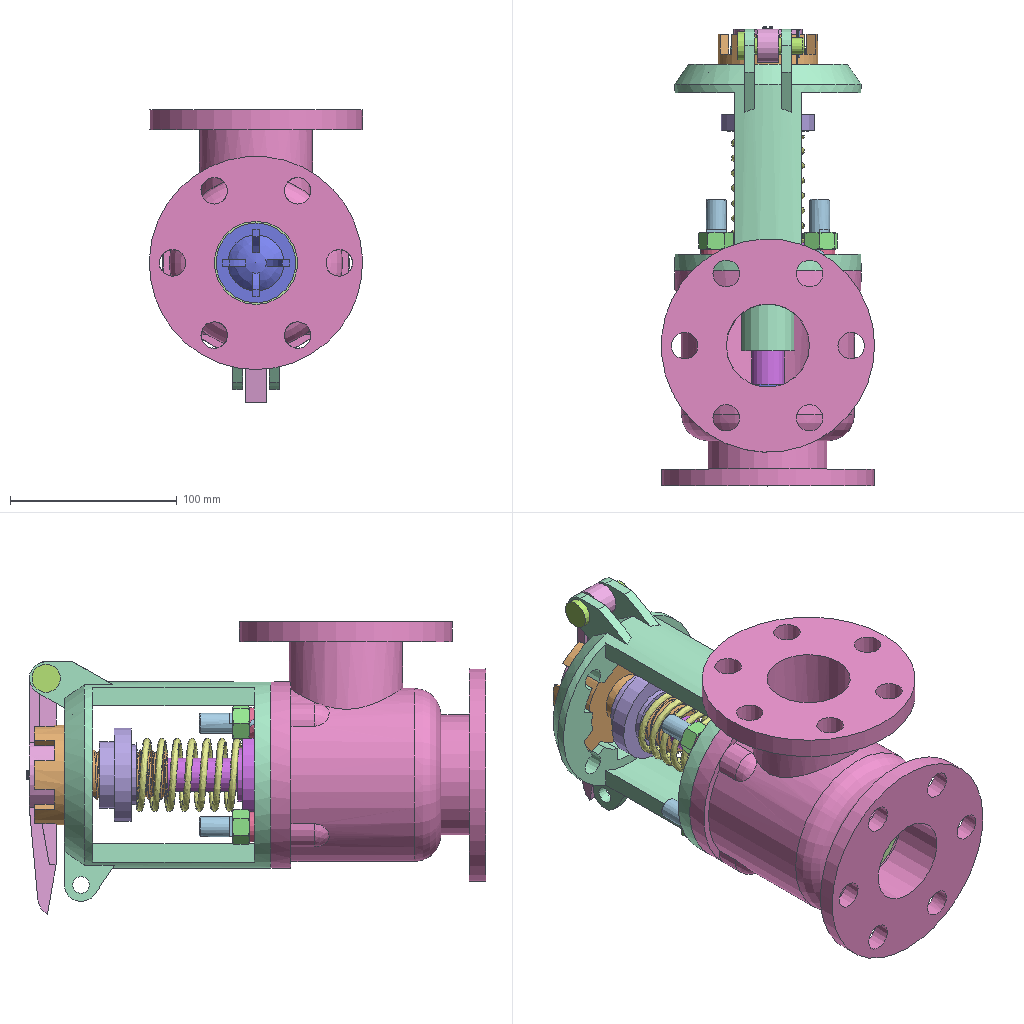Assembly | NX | 17 different items | 26 placed | box 128 x 276 x 176 mm
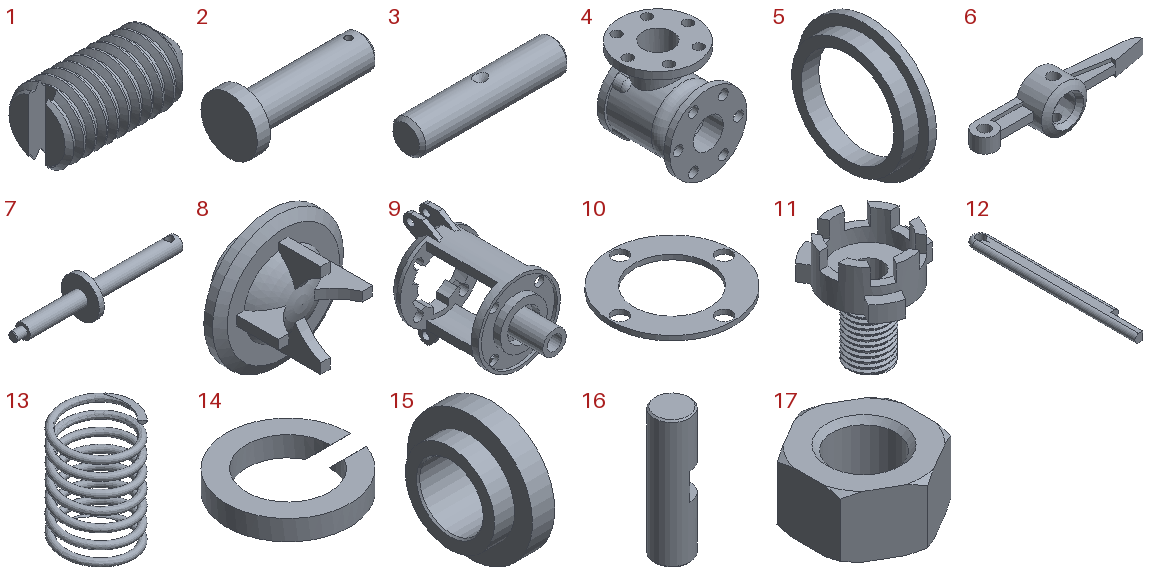Parts list (item | quantity | size | volume | features):
1 | x1 | 12 x 6 x 6 mm | 246.547 mm3 | features DATUM_CSYS 3, SKETCH 2, CHAMFER 1, EXTRUDE 1, SWP104 1, THREADS 1
2 | x1 | 40 x 17 x 17 mm | 3696 mm3 | features DATUM_CSYS 3, SKETCH 2, EXTRUDE 1, SWP104 1
3 | x1 | 45 x 10 x 10 mm | 3498 mm3 | features DATUM_CSYS 4, SKETCH 3, SWP104 2
4 | x1 | 128 x 148 x 156 mm | 660287 mm3 | features EXTRUDE 6, DATUM_CSYS 5, SIMPLE HOLE 4, SKETCH 4, SYMBOLIC_THREAD 4, BLEND 1, HOLE PACKAGE 1, REPLACE_FACE 1, SWP104 1, UNITE 1
5 | x1 | 12 x 68 x 68 mm | 12689 mm3 | features DATUM_CSYS 2, SKETCH 1, SWP104 1
6 | x1 | 151.676 x 27.098 x 41 mm | 35006 mm3 | features EXTRUDE 7, DATUM_CSYS 5, SKETCH 4, SWP104 3, REPLACE_FACE 2, CHAMFER 1, UNITE 1
7 | x1 | 223 x 52 x 52 mm | 79707 mm3 | features DATUM_CSYS 3, SKETCH 2, CHAMFER 1, EXTRUDE 1, HOLE PACKAGE 1, SIMPLE HOLE 1, SWP104 1, SYMBOLIC_THREAD 1
8 | x1 | 56 x 35 x 56 mm | 23365 mm3 | features DATUM_CSYS 3, EXTRACT_STRING 2, EXTRUDE 2, SKETCH 2, HOLE PACKAGE 1, Instance Feature 1, Pattern Feature 1, SIMPLE HOLE 1, SWP104 1
9 | x1 | 112 x 193 x 144 mm | 268281 mm3 | features EXTRUDE 8, DATUM_CSYS 6, SKETCH 5, EXTRACT_STRING 4, CHAMFER 1, Instance Feature 1, Mirror Feature 1, REPLACE_FACE 1, SWP104 1, UNITE 1
10 | x1 | 104 x 104 x 4 mm | 18988 mm3 | features DATUM_CSYS 2, EXTRUDE 1, SKETCH 1
11 | x1 | 68 x 73.498 x 80 mm | 58295 mm3 | features EXTRUDE 6, DATUM_CSYS 2, SKETCH 1, THREADS 1
12 | x1 | 2 x 21 x 1 mm | 32.529 mm3 | features DATUM_CSYS 2, EXTRUDE 2, BLEND 1, SKETCH 1
13 | x1 | 43.994 x 43.994 x 64 mm | 11223 mm3 | features DATUM_CSYS 2, SKETCH 2, DATUM_ON_PATH 1, EXTRUDE 1, HELIX 1, LINE 1, SKIN 1
14 | x4 | 18.3 x 18.3 x 3 mm | 406.803 mm3 | features DATUM_CSYS 3, EXTRUDE 2, SKETCH 2
15 | x1 | 22 x 56 x 56 mm | 24872 mm3 | features DATUM_CSYS 2, HOLE PACKAGE 1, SIMPLE HOLE 1, SKETCH 1, SWP104 1, SYMBOLIC_THREAD 1
16 | x4 | 12 x 12 x 43 mm | 4345 mm3 | features DATUM_CSYS 2, CHAMFER 1, CYLINDER 1, EXTRUDE 1, SKETCH 1
17 | x4 | 18 x 20.785 x 10 mm | 1943 mm3 | features DATUM_CSYS 3, EXTRACT_FACE 2, EXTRACT_STRING 2, SKETCH 2, SWP104 2, EXTRUDE 1, HOLE PACKAGE 1, Instance Feature 1, Mirror Feature 1, SIMPLE HOLE 1, SYMBOLIC_THREAD 1
Mates (type | each side: item.copy, entity, surface, feature):
Fix | 4.1 component
Touch | 5.1 face cylinder Revolve(2) | 4.1 face cylinder Revolve(2)
Touch | 5.1 face plane Revolve(2) | 4.1 face plane Revolve(2)
AlignLock | 5.1 face cylinder Revolve(2) | 4.1 face cylinder Revolve(2)
Touch | 8.1 face cylinder Ø16 Hole(6) | 5.1 face cylinder Revolve(2)
Touch | 8.1 face cone Revolve(2) | 5.1 face cone Revolve(2)
AlignLock | 8.1 face cylinder Revolve(2) | 4.1 face cylinder Revolve(2)
Touch | 10.1 face cylinder Extrude(2) | 4.1 face cylinder M12 x 1.75 Threaded Hole(15) | 2 times
Touch | 10.1 face plane Extrude(2) | 4.1 face plane Revolve(2)
Touch | 9.1 face cylinder Revolve(2) | 4.1 face cylinder Revolve(2)
Touch | 9.1 face plane Revolve(2) | 4.1 face plane Revolve(2)
AlignLock | 9.1 face cylinder Revolve(2) | 4.1 face cylinder Revolve(2)
Touch | 7.1 face cylinder Revolve(2) | 9.1 face cylinder Revolve(2)
Touch | 7.1 face plane Revolve(2) | 8.1 face plane Revolve(2)
Touch | 13.1 line | 9.1 face cylinder Revolve(2)
Touch | 13.1 face plane Extrude(5) | 7.1 face plane Revolve(2)
Angle | 13.1 face plane Swept(3) | 4.1 face plane Extrude(6)
Touch | 16.1 face cylinder Cylinder(1) | 9.1 face cylinder Extrude(13)
Touch | 16.1 face plane Cylinder(1) | 4.1 face plane Revolve(2)
AlignLock | 16.1 face cylinder Cylinder(1) | 9.1 face cylinder Extrude(13)
Touch | 14.1 face cylinder Extrude(2) | 16.1 face cylinder Cylinder(1)
Touch | 14.1 face plane Extrude(2) | 9.1 face plane Revolve(2)
Angle | 14.1 face plane Extrude(4) | 4.1 face plane Extrude(4)
Touch | 17.1 face cylinder M12 x 1.75 Threaded Hole(7) | 16.1 face cylinder Cylinder(1)
Touch | 17.1 face plane Extrude(2) | 14.1 face plane Extrude(2)
Angle | 17.1 face plane Extrude(2) | 9.1 face plane Extrude(16)
Bond | 9.1 component | assembly component
Bond | 16.1 component | assembly component | 4 times
Bond | 14.1 component | assembly component | 4 times
Bond | 17.1 component | assembly component | 4 times
CircularPattern | assembly axis | assembly csys | assembly csys | assembly csys | assembly csys | 3 times
Touch | 15.1 line | 7.1 face cylinder Revolve(2)
Touch | 15.1 face plane Revolve(2) | 13.1 face plane Extrude(5)
AlignLock | 15.1 face cylinder Revolve(2) | 9.1 face cylinder Revolve(2)
Distance | 11.1 face plane Extrude(4) | 9.1 face plane Revolve(2)
AlignLock | 7.1 face cylinder Revolve(2) | 11.1 face cylinder Extrude(5)
AlignLock | 7.1 face cylinder Revolve(2) | 9.1 face cylinder Revolve(2)
AlignLock | 3.1 face cylinder Revolve(2) | 7.1 face cylinder Extrude(5)
Distance | 3.1 face plane Revolve(2) | 7.1 face cylinder Revolve(2)
Touch | 6.1 face cone Revolve(18) | 11.1 face cylinder Extrude(3)
Parallel | 6.1 face plane Extrude(2) | 9.1 face plane Mirror Feature(8)
Touch | 6.1 face cylinder Extrude(15) | 3.1 face cylinder Revolve(2)
Touch | 2.1 face cylinder Revolve(2) | 9.1 face cylinder Extrude(7)
Touch | 2.1 face plane Revolve(2) | 9.1 face plane Extrude(7)
AlignLock | 2.1 face cylinder Revolve(2) | 9.1 face cylinder Mirror Feature(8)
Distance | 12.1 face plane Extrude(2) | 2.1 face cylinder Extrude(4)
Distance | 12.1 face surfaceofrevolution Edge Blend(4) | 2.1 face cylinder Extrude(4)
Distance | 12.1 face plane Extrude(2) | 9.1 face plane Revolve(2)
Parallel | 1.1 face plane Extrude(6) | 6.1 face plane Extrude(2)
Touch | 1.1 face cylinder Threads(4) | 7.1 face cylinder M6 x 1.0 Threaded Hole(6)
Touch | 1.1 face cone Revolve(2) | 3.1 face cone Revolve(7)
Parallel | 12.1 face plane Extrude(2) | 9.1 face plane Mirror Feature(8)